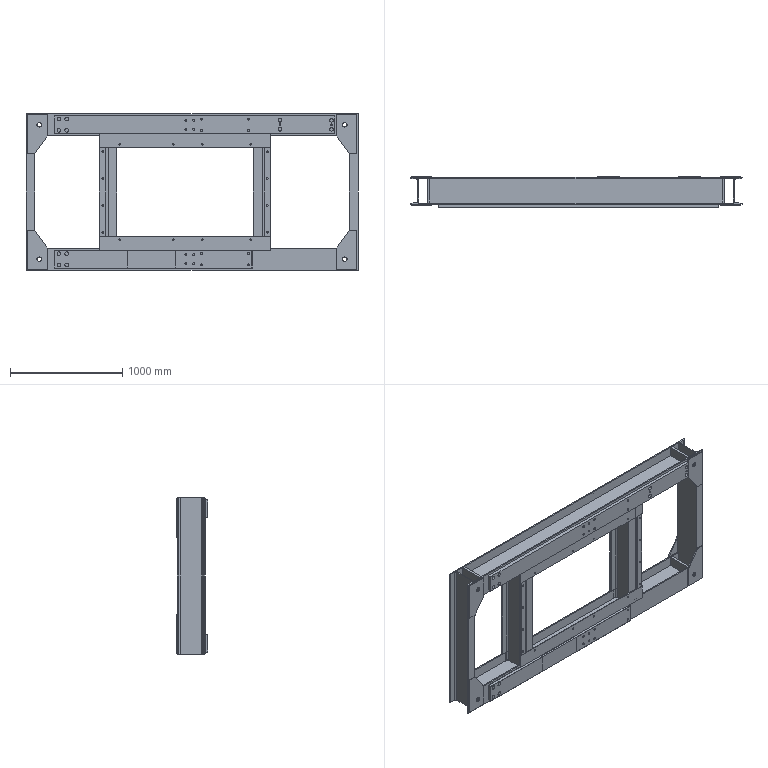Part | NX | features BREP 14, DATUM_CSYS 3, SKETCH 3, LINKED_FACE 1, REPLACE_FACE 1 | 34 solids | 420 faces | box 2963 x 280 x 1400 mm | volume 109819651 mm3 | plane 272 | cylinder 148 | commonest cylinder face diameters 18 x32 40 x32 12 x28 32 x24 14 x16 24 x12